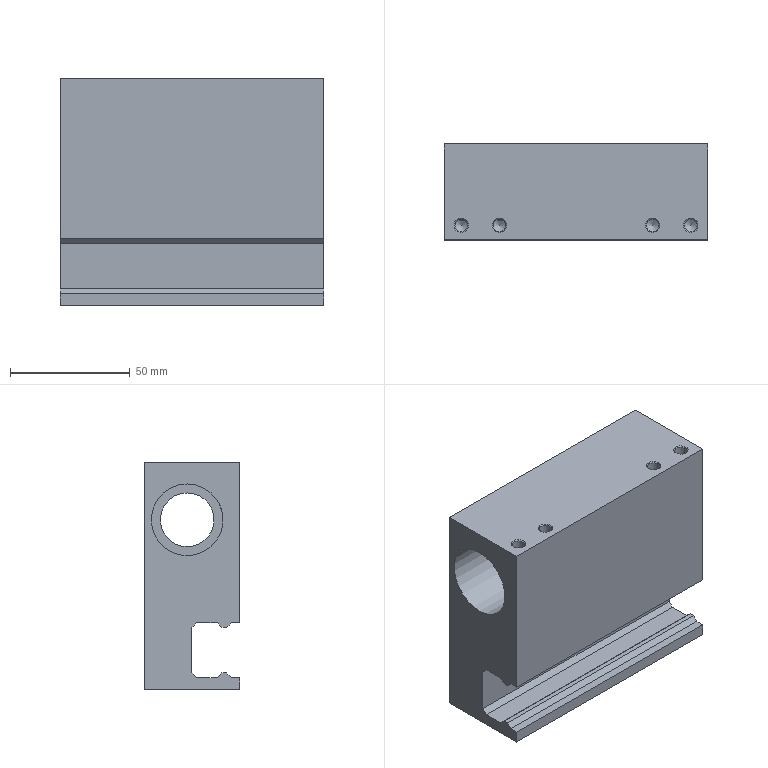Part | NX | features SIMPLE HOLE 14, SYMBOLIC_THREAD 13, DATUM_CSYS 6, HOLE PACKAGE 5, SKETCH 5, EXTRUDE 2, SUBTRACT 1 | 1 solid | 61 faces | box 110 x 40 x 95 mm | volume 303623 mm3 | cone 24 | plane 22 | cylinder 15 | commonest cylinder face diameters 5.2 x12 22.5 x1 29 x1 30 x1
STEP:
#1=CARTESIAN_POINT('',(-55.,-3.5,11.5));
#2=VERTEX_POINT('',#1);
#3=CARTESIAN_POINT('',(55.,-3.5,11.5));
#4=VERTEX_POINT('',#3);
#5=CARTESIAN_POINT('',(55.,-3.5,11.5));
#6=DIRECTION('',(-1.,0.,0.));
#7=VECTOR('',#6,1000.);
#8=LINE('',#5,#7);
#9=EDGE_CURVE('',#2,#4,#8,.F.);
#10=ORIENTED_EDGE('',*,*,#9,.T.);
#11=CARTESIAN_POINT('',(55.,-3.5,78.5));
#12=VERTEX_POINT('',#11);
#13=CARTESIAN_POINT('',(55.,-3.5,78.5));
#14=DIRECTION('',(0.,0.,-1.));
#15=VECTOR('',#14,1000.);
#16=LINE('',#13,#15);
#17=EDGE_CURVE('',#12,#4,#16,.T.);
#18=ORIENTED_EDGE('',*,*,#17,.F.);
#19=CARTESIAN_POINT('',(-55.,-3.5,78.5));
#20=VERTEX_POINT('',#19);
#21=CARTESIAN_POINT('',(55.,-3.5,78.5));
#22=DIRECTION('',(-1.,0.,0.));
#23=VECTOR('',#22,1000.);
#24=LINE('',#21,#23);
#25=EDGE_CURVE('',#12,#20,#24,.T.);
#26=ORIENTED_EDGE('',*,*,#25,.T.);
#27=CARTESIAN_POINT('',(-55.,-3.5,78.5));
#28=DIRECTION('',(0.,0.,-1.));
#29=VECTOR('',#28,1000.);
#30=LINE('',#27,#29);
#31=EDGE_CURVE('',#20,#2,#30,.T.);
#32=ORIENTED_EDGE('',*,*,#31,.T.);
#33=EDGE_LOOP('',(#10,#18,#26,#32));
#34=FACE_BOUND('',#33,.T.);
#35=CARTESIAN_POINT('',(55.,-3.5,78.5));
#36=DIRECTION('',(0.,1.,0.));
#37=DIRECTION('',(0.,0.,1.));
#38=AXIS2_PLACEMENT_3D('',#35,#36,#37);
#39=PLANE('',#38);
#40=ADVANCED_FACE('',(#34),#39,.F.);
#41=CARTESIAN_POINT('',(55.,-3.5,-11.5));
#42=VERTEX_POINT('',#41);
#43=CARTESIAN_POINT('',(-55.,-3.5,-11.5));
#44=VERTEX_POINT('',#43);
#45=CARTESIAN_POINT('',(55.,-3.5,-11.5));
#46=DIRECTION('',(1.,0.,0.));
#47=VECTOR('',#46,1000.);
#48=LINE('',#45,#47);
#49=EDGE_CURVE('',#42,#44,#48,.F.);
#50=ORIENTED_EDGE('',*,*,#49,.T.);
#51=CARTESIAN_POINT('',(-55.,-3.5,-16.5));
#52=VERTEX_POINT('',#51);
#53=CARTESIAN_POINT('',(-55.,-3.5,78.5));
#54=DIRECTION('',(0.,0.,-1.));
#55=VECTOR('',#54,1000.);
#56=LINE('',#53,#55);
#57=EDGE_CURVE('',#44,#52,#56,.T.);
#58=ORIENTED_EDGE('',*,*,#57,.T.);
#59=CARTESIAN_POINT('',(55.,-3.5,-16.5));
#60=VERTEX_POINT('',#59);
#61=CARTESIAN_POINT('',(55.,-3.5,-16.5));
#62=DIRECTION('',(-1.,0.,0.));
#63=VECTOR('',#62,1000.);
#64=LINE('',#61,#63);
#65=EDGE_CURVE('',#60,#52,#64,.T.);
#66=ORIENTED_EDGE('',*,*,#65,.F.);
#67=CARTESIAN_POINT('',(55.,-3.5,78.5));
#68=DIRECTION('',(0.,0.,-1.));
#69=VECTOR('',#68,1000.);
#70=LINE('',#67,#69);
#71=EDGE_CURVE('',#42,#60,#70,.T.);
#72=ORIENTED_EDGE('',*,*,#71,.F.);
#73=EDGE_LOOP('',(#50,#58,#66,#72));
#74=FACE_BOUND('',#73,.T.);
#75=CARTESIAN_POINT('',(55.,-3.5,78.5));
#76=DIRECTION('',(0.,1.,0.));
#77=DIRECTION('',(0.,0.,1.));
#78=AXIS2_PLACEMENT_3D('',#75,#76,#77);
#79=PLANE('',#78);
#80=ADVANCED_FACE('',(#74),#79,.F.);
#81=CARTESIAN_POINT('',(55.,18.5,69.));
#82=VERTEX_POINT('',#81);
#83=CARTESIAN_POINT('',(55.,18.5,54.5));
#84=DIRECTION('',(-1.,0.,0.));
#85=DIRECTION('',(0.,0.,1.));
#86=AXIS2_PLACEMENT_3D('',#83,#84,#85);
#87=CIRCLE('',#86,14.5);
#88=EDGE_CURVE('',#82,#82,#87,.T.);
#89=ORIENTED_EDGE('',*,*,#88,.T.);
#90=EDGE_LOOP('',(#89));
#91=FACE_BOUND('',#90,.T.);
#92=ORIENTED_EDGE('',*,*,#17,.T.);
#93=CARTESIAN_POINT('',(55.,0.,11.5));
#94=VERTEX_POINT('',#93);
#95=CARTESIAN_POINT('',(55.,18.5,11.5));
#96=DIRECTION('',(0.,1.,0.));
#97=VECTOR('',#96,1000.);
#98=LINE('',#95,#97);
#99=EDGE_CURVE('',#94,#4,#98,.F.);
#100=ORIENTED_EDGE('',*,*,#99,.F.);
#101=CARTESIAN_POINT('',(55.,2.,9.5));
#102=VERTEX_POINT('',#101);
#103=CARTESIAN_POINT('',(55.,-12.25,23.75));
#104=DIRECTION('',(0.,0.7071,-0.7071));
#105=VECTOR('',#104,1000.);
#106=LINE('',#103,#105);
#107=EDGE_CURVE('',#102,#94,#106,.F.);
#108=ORIENTED_EDGE('',*,*,#107,.F.);
#109=CARTESIAN_POINT('',(55.,4.,9.5));
#110=VERTEX_POINT('',#109);
#111=CARTESIAN_POINT('',(55.,18.5,9.5));
#112=DIRECTION('',(0.,1.,0.));
#113=VECTOR('',#112,1000.);
#114=LINE('',#111,#113);
#115=EDGE_CURVE('',#110,#102,#114,.F.);
#116=ORIENTED_EDGE('',*,*,#115,.F.);
#117=CARTESIAN_POINT('',(55.,6.,11.5));
#118=VERTEX_POINT('',#117);
#119=CARTESIAN_POINT('',(55.,33.75,39.25));
#120=DIRECTION('',(0.,0.7071,0.7071));
#121=VECTOR('',#120,1000.);
#122=LINE('',#119,#121);
#123=EDGE_CURVE('',#118,#110,#122,.F.);
#124=ORIENTED_EDGE('',*,*,#123,.F.);
#125=CARTESIAN_POINT('',(55.,14.5,11.5));
#126=VERTEX_POINT('',#125);
#127=CARTESIAN_POINT('',(55.,18.5,11.5));
#128=DIRECTION('',(0.,1.,0.));
#129=VECTOR('',#128,1000.);
#130=LINE('',#127,#129);
#131=EDGE_CURVE('',#126,#118,#130,.F.);
#132=ORIENTED_EDGE('',*,*,#131,.F.);
#133=CARTESIAN_POINT('',(55.,16.5,9.5));
#134=VERTEX_POINT('',#133);
#135=CARTESIAN_POINT('',(55.,-5.,31.));
#136=DIRECTION('',(0.,0.7071,-0.7071));
#137=VECTOR('',#136,1000.);
#138=LINE('',#135,#137);
#139=EDGE_CURVE('',#134,#126,#138,.F.);
#140=ORIENTED_EDGE('',*,*,#139,.F.);
#141=CARTESIAN_POINT('',(55.,16.5,-9.5));
#142=VERTEX_POINT('',#141);
#143=CARTESIAN_POINT('',(55.,16.5,54.5));
#144=DIRECTION('',(0.,0.,-1.));
#145=VECTOR('',#144,1000.);
#146=LINE('',#143,#145);
#147=EDGE_CURVE('',#142,#134,#146,.F.);
#148=ORIENTED_EDGE('',*,*,#147,.F.);
#149=CARTESIAN_POINT('',(55.,14.5,-11.5));
#150=VERTEX_POINT('',#149);
#151=CARTESIAN_POINT('',(55.,49.5,23.5));
#152=DIRECTION('',(0.,-0.7071,-0.7071));
#153=VECTOR('',#152,1000.);
#154=LINE('',#151,#153);
#155=EDGE_CURVE('',#150,#142,#154,.F.);
#156=ORIENTED_EDGE('',*,*,#155,.F.);
#157=CARTESIAN_POINT('',(55.,6.,-11.5));
#158=VERTEX_POINT('',#157);
#159=CARTESIAN_POINT('',(55.,18.5,-11.5));
#160=DIRECTION('',(0.,-1.,0.));
#161=VECTOR('',#160,1000.);
#162=LINE('',#159,#161);
#163=EDGE_CURVE('',#158,#150,#162,.F.);
#164=ORIENTED_EDGE('',*,*,#163,.F.);
#165=CARTESIAN_POINT('',(55.,4.,-9.5));
#166=VERTEX_POINT('',#165);
#167=CARTESIAN_POINT('',(55.,-20.75,15.25));
#168=DIRECTION('',(0.,-0.7071,0.7071));
#169=VECTOR('',#168,1000.);
#170=LINE('',#167,#169);
#171=EDGE_CURVE('',#166,#158,#170,.F.);
#172=ORIENTED_EDGE('',*,*,#171,.F.);
#173=CARTESIAN_POINT('',(55.,2.,-9.5));
#174=VERTEX_POINT('',#173);
#175=CARTESIAN_POINT('',(55.,18.5,-9.5));
#176=DIRECTION('',(0.,-1.,0.));
#177=VECTOR('',#176,1000.);
#178=LINE('',#175,#177);
#179=EDGE_CURVE('',#174,#166,#178,.F.);
#180=ORIENTED_EDGE('',*,*,#179,.F.);
#181=CARTESIAN_POINT('',(55.,0.,-11.5));
#182=VERTEX_POINT('',#181);
#183=CARTESIAN_POINT('',(55.,42.25,30.75));
#184=DIRECTION('',(0.,-0.7071,-0.7071));
#185=VECTOR('',#184,1000.);
#186=LINE('',#183,#185);
#187=EDGE_CURVE('',#182,#174,#186,.F.);
#188=ORIENTED_EDGE('',*,*,#187,.F.);
#189=CARTESIAN_POINT('',(55.,18.5,-11.5));
#190=DIRECTION('',(0.,-1.,0.));
#191=VECTOR('',#190,1000.);
#192=LINE('',#189,#191);
#193=EDGE_CURVE('',#42,#182,#192,.F.);
#194=ORIENTED_EDGE('',*,*,#193,.F.);
#195=ORIENTED_EDGE('',*,*,#71,.T.);
#196=CARTESIAN_POINT('',(55.,36.5,-16.5));
#197=VERTEX_POINT('',#196);
#198=CARTESIAN_POINT('',(55.,-3.5,-16.5));
#199=DIRECTION('',(0.,1.,0.));
#200=VECTOR('',#199,1000.);
#201=LINE('',#198,#200);
#202=EDGE_CURVE('',#60,#197,#201,.T.);
#203=ORIENTED_EDGE('',*,*,#202,.T.);
#204=CARTESIAN_POINT('',(55.,36.5,78.5));
#205=VERTEX_POINT('',#204);
#206=CARTESIAN_POINT('',(55.,36.5,-16.5));
#207=DIRECTION('',(0.,0.,1.));
#208=VECTOR('',#207,1000.);
#209=LINE('',#206,#208);
#210=EDGE_CURVE('',#197,#205,#209,.T.);
#211=ORIENTED_EDGE('',*,*,#210,.T.);
#212=CARTESIAN_POINT('',(55.,36.5,78.5));
#213=DIRECTION('',(0.,-1.,0.));
#214=VECTOR('',#213,1000.);
#215=LINE('',#212,#214);
#216=EDGE_CURVE('',#205,#12,#215,.T.);
#217=ORIENTED_EDGE('',*,*,#216,.T.);
#218=EDGE_LOOP('',(#92,#100,#108,#116,#124,#132,#140,#148,#156,#164,#172,#180,#188,#194,#195,#203,#211,#217));
#219=FACE_BOUND('',#218,.T.);
#220=CARTESIAN_POINT('',(55.,18.5,54.5));
#221=DIRECTION('',(1.,0.,0.));
#222=DIRECTION('',(0.,0.,-1.));
#223=AXIS2_PLACEMENT_3D('',#220,#221,#222);
#224=PLANE('',#223);
#225=ADVANCED_FACE('',(#91,#219),#224,.T.);
#226=CARTESIAN_POINT('',(-55.,18.5,39.5));
#227=VERTEX_POINT('',#226);
#228=CARTESIAN_POINT('',(-55.,18.5,54.5));
#229=DIRECTION('',(1.,0.,0.));
#230=DIRECTION('',(0.,0.,-1.));
#231=AXIS2_PLACEMENT_3D('',#228,#229,#230);
#232=CIRCLE('',#231,15.);
#233=EDGE_CURVE('',#227,#227,#232,.T.);
#234=ORIENTED_EDGE('',*,*,#233,.T.);
#235=EDGE_LOOP('',(#234));
#236=FACE_BOUND('',#235,.T.);
#237=CARTESIAN_POINT('',(-55.,0.,11.5));
#238=VERTEX_POINT('',#237);
#239=CARTESIAN_POINT('',(-55.,18.5,11.5));
#240=DIRECTION('',(0.,1.,0.));
#241=VECTOR('',#240,1000.);
#242=LINE('',#239,#241);
#243=EDGE_CURVE('',#238,#2,#242,.F.);
#244=ORIENTED_EDGE('',*,*,#243,.T.);
#245=ORIENTED_EDGE('',*,*,#31,.F.);
#246=CARTESIAN_POINT('',(-55.,36.5,78.5));
#247=VERTEX_POINT('',#246);
#248=CARTESIAN_POINT('',(-55.,36.5,78.5));
#249=DIRECTION('',(0.,-1.,0.));
#250=VECTOR('',#249,1000.);
#251=LINE('',#248,#250);
#252=EDGE_CURVE('',#247,#20,#251,.T.);
#253=ORIENTED_EDGE('',*,*,#252,.F.);
#254=CARTESIAN_POINT('',(-55.,36.5,-16.5));
#255=VERTEX_POINT('',#254);
#256=CARTESIAN_POINT('',(-55.,36.5,-16.5));
#257=DIRECTION('',(0.,0.,1.));
#258=VECTOR('',#257,1000.);
#259=LINE('',#256,#258);
#260=EDGE_CURVE('',#255,#247,#259,.T.);
#261=ORIENTED_EDGE('',*,*,#260,.F.);
#262=CARTESIAN_POINT('',(-55.,-3.5,-16.5));
#263=DIRECTION('',(0.,1.,0.));
#264=VECTOR('',#263,1000.);
#265=LINE('',#262,#264);
#266=EDGE_CURVE('',#52,#255,#265,.T.);
#267=ORIENTED_EDGE('',*,*,#266,.F.);
#268=ORIENTED_EDGE('',*,*,#57,.F.);
#269=CARTESIAN_POINT('',(-55.,0.,-11.5));
#270=VERTEX_POINT('',#269);
#271=CARTESIAN_POINT('',(-55.,18.5,-11.5));
#272=DIRECTION('',(0.,-1.,0.));
#273=VECTOR('',#272,1000.);
#274=LINE('',#271,#273);
#275=EDGE_CURVE('',#44,#270,#274,.F.);
#276=ORIENTED_EDGE('',*,*,#275,.T.);
#277=CARTESIAN_POINT('',(-55.,2.,-9.5));
#278=VERTEX_POINT('',#277);
#279=CARTESIAN_POINT('',(-55.,42.25,30.75));
#280=DIRECTION('',(0.,-0.7071,-0.7071));
#281=VECTOR('',#280,1000.);
#282=LINE('',#279,#281);
#283=EDGE_CURVE('',#270,#278,#282,.F.);
#284=ORIENTED_EDGE('',*,*,#283,.T.);
#285=CARTESIAN_POINT('',(-55.,4.,-9.5));
#286=VERTEX_POINT('',#285);
#287=CARTESIAN_POINT('',(-55.,18.5,-9.5));
#288=DIRECTION('',(0.,-1.,0.));
#289=VECTOR('',#288,1000.);
#290=LINE('',#287,#289);
#291=EDGE_CURVE('',#278,#286,#290,.F.);
#292=ORIENTED_EDGE('',*,*,#291,.T.);
#293=CARTESIAN_POINT('',(-55.,6.,-11.5));
#294=VERTEX_POINT('',#293);
#295=CARTESIAN_POINT('',(-55.,-20.75,15.25));
#296=DIRECTION('',(0.,-0.7071,0.7071));
#297=VECTOR('',#296,1000.);
#298=LINE('',#295,#297);
#299=EDGE_CURVE('',#286,#294,#298,.F.);
#300=ORIENTED_EDGE('',*,*,#299,.T.);
#301=CARTESIAN_POINT('',(-55.,14.5,-11.5));
#302=VERTEX_POINT('',#301);
#303=CARTESIAN_POINT('',(-55.,18.5,-11.5));
#304=DIRECTION('',(0.,-1.,0.));
#305=VECTOR('',#304,1000.);
#306=LINE('',#303,#305);
#307=EDGE_CURVE('',#294,#302,#306,.F.);
#308=ORIENTED_EDGE('',*,*,#307,.T.);
#309=CARTESIAN_POINT('',(-55.,16.5,-9.5));
#310=VERTEX_POINT('',#309);
#311=CARTESIAN_POINT('',(-55.,49.5,23.5));
#312=DIRECTION('',(0.,-0.7071,-0.7071));
#313=VECTOR('',#312,1000.);
#314=LINE('',#311,#313);
#315=EDGE_CURVE('',#302,#310,#314,.F.);
#316=ORIENTED_EDGE('',*,*,#315,.T.);
#317=CARTESIAN_POINT('',(-55.,16.5,9.5));
#318=VERTEX_POINT('',#317);
#319=CARTESIAN_POINT('',(-55.,16.5,54.5));
#320=DIRECTION('',(0.,0.,-1.));
#321=VECTOR('',#320,1000.);
#322=LINE('',#319,#321);
#323=EDGE_CURVE('',#310,#318,#322,.F.);
#324=ORIENTED_EDGE('',*,*,#323,.T.);
#325=CARTESIAN_POINT('',(-55.,14.5,11.5));
#326=VERTEX_POINT('',#325);
#327=CARTESIAN_POINT('',(-55.,-5.,31.));
#328=DIRECTION('',(0.,0.7071,-0.7071));
#329=VECTOR('',#328,1000.);
#330=LINE('',#327,#329);
#331=EDGE_CURVE('',#318,#326,#330,.F.);
#332=ORIENTED_EDGE('',*,*,#331,.T.);
#333=CARTESIAN_POINT('',(-55.,6.,11.5));
#334=VERTEX_POINT('',#333);
#335=CARTESIAN_POINT('',(-55.,18.5,11.5));
#336=DIRECTION('',(0.,1.,0.));
#337=VECTOR('',#336,1000.);
#338=LINE('',#335,#337);
#339=EDGE_CURVE('',#326,#334,#338,.F.);
#340=ORIENTED_EDGE('',*,*,#339,.T.);
#341=CARTESIAN_POINT('',(-55.,4.,9.5));
#342=VERTEX_POINT('',#341);
#343=CARTESIAN_POINT('',(-55.,33.75,39.25));
#344=DIRECTION('',(0.,0.7071,0.7071));
#345=VECTOR('',#344,1000.);
#346=LINE('',#343,#345);
#347=EDGE_CURVE('',#334,#342,#346,.F.);
#348=ORIENTED_EDGE('',*,*,#347,.T.);
#349=CARTESIAN_POINT('',(-55.,2.,9.5));
#350=VERTEX_POINT('',#349);
#351=CARTESIAN_POINT('',(-55.,18.5,9.5));
#352=DIRECTION('',(0.,1.,0.));
#353=VECTOR('',#352,1000.);
#354=LINE('',#351,#353);
#355=EDGE_CURVE('',#342,#350,#354,.F.);
#356=ORIENTED_EDGE('',*,*,#355,.T.);
#357=CARTESIAN_POINT('',(-55.,-12.25,23.75));
#358=DIRECTION('',(0.,0.7071,-0.7071));
#359=VECTOR('',#358,1000.);
#360=LINE('',#357,#359);
#361=EDGE_CURVE('',#350,#238,#360,.F.);
#362=ORIENTED_EDGE('',*,*,#361,.T.);
#363=EDGE_LOOP('',(#244,#245,#253,#261,#267,#268,#276,#284,#292,#300,#308,#316,#324,#332,#340,#348,#356,#362));
#364=FACE_BOUND('',#363,.T.);
#365=CARTESIAN_POINT('',(-55.,18.5,54.5));
#366=DIRECTION('',(1.,0.,0.));
#367=DIRECTION('',(0.,0.,-1.));
#368=AXIS2_PLACEMENT_3D('',#365,#366,#367);
#369=PLANE('',#368);
#370=ADVANCED_FACE('',(#236,#364),#369,.F.);
#371=CARTESIAN_POINT('',(43.,22.5,-16.5));
#372=VERTEX_POINT('',#371);
#373=CARTESIAN_POINT('',(40.,22.5,-16.5));
#374=DIRECTION('',(0.,0.,1.));
#375=DIRECTION('',(1.,0.,0.));
#376=AXIS2_PLACEMENT_3D('',#373,#374,#375);
#377=CIRCLE('',#376,3.);
#378=EDGE_CURVE('',#372,#372,#377,.T.);
#379=ORIENTED_EDGE('',*,*,#378,.T.);
#380=EDGE_LOOP('',(#379));
#381=FACE_BOUND('',#380,.T.);
#382=CARTESIAN_POINT('',(17.,22.5,-16.5));
#383=VERTEX_POINT('',#382);
#384=CARTESIAN_POINT('',(14.,22.5,-16.5));
#385=DIRECTION('',(0.,0.,1.));
#386=DIRECTION('',(1.,0.,0.));
#387=AXIS2_PLACEMENT_3D('',#384,#385,#386);
#388=CIRCLE('',#387,3.);
#389=EDGE_CURVE('',#383,#383,#388,.T.);
#390=ORIENTED_EDGE('',*,*,#389,.T.);
#391=EDGE_LOOP('',(#390));
#392=FACE_BOUND('',#391,.T.);
#393=CARTESIAN_POINT('',(-11.,22.5,-16.5));
#394=VERTEX_POINT('',#393);
#395=CARTESIAN_POINT('',(-14.,22.5,-16.5));
#396=DIRECTION('',(0.,0.,1.));
#397=DIRECTION('',(1.,0.,0.));
#398=AXIS2_PLACEMENT_3D('',#395,#396,#397);
#399=CIRCLE('',#398,3.);
#400=EDGE_CURVE('',#394,#394,#399,.T.);
#401=ORIENTED_EDGE('',*,*,#400,.T.);
#402=EDGE_LOOP('',(#401));
#403=FACE_BOUND('',#402,.T.);
#404=CARTESIAN_POINT('',(-37.,22.5,-16.5));
#405=VERTEX_POINT('',#404);
#406=CARTESIAN_POINT('',(-40.,22.5,-16.5));
#407=DIRECTION('',(0.,0.,1.));
#408=DIRECTION('',(1.,0.,0.));
#409=AXIS2_PLACEMENT_3D('',#406,#407,#408);
#410=CIRCLE('',#409,3.);
#411=EDGE_CURVE('',#405,#405,#410,.T.);
#412=ORIENTED_EDGE('',*,*,#411,.T.);
#413=EDGE_LOOP('',(#412));
#414=FACE_BOUND('',#413,.T.);
#415=ORIENTED_EDGE('',*,*,#266,.T.);
#416=CARTESIAN_POINT('',(55.,36.5,-16.5));
#417=DIRECTION('',(-1.,0.,0.));
#418=VECTOR('',#417,1000.);
#419=LINE('',#416,#418);
#420=EDGE_CURVE('',#197,#255,#419,.T.);
#421=ORIENTED_EDGE('',*,*,#420,.F.);
#422=ORIENTED_EDGE('',*,*,#202,.F.);
#423=ORIENTED_EDGE('',*,*,#65,.T.);
#424=EDGE_LOOP('',(#415,#421,#422,#423));
#425=FACE_BOUND('',#424,.T.);
#426=CARTESIAN_POINT('',(55.,-3.5,-16.5));
#427=DIRECTION('',(0.,0.,1.));
#428=DIRECTION('',(1.,0.,0.));
#429=AXIS2_PLACEMENT_3D('',#426,#427,#428);
#430=PLANE('',#429);
#431=ADVANCED_FACE('',(#381,#392,#403,#414,#425),#430,.F.);
#432=CARTESIAN_POINT('',(46.,36.5,33.5));
#433=VERTEX_POINT('',#432);
#434=CARTESIAN_POINT('',(46.,36.5,36.5));
#435=DIRECTION('',(0.,-1.,0.));
#436=DIRECTION('',(0.,0.,-1.));
#437=AXIS2_PLACEMENT_3D('',#434,#435,#436);
#438=CIRCLE('',#437,3.);
#439=EDGE_CURVE('',#433,#433,#438,.T.);
#440=ORIENTED_EDGE('',*,*,#439,.T.);
#441=EDGE_LOOP('',(#440));
#442=FACE_BOUND('',#441,.T.);
#443=CARTESIAN_POINT('',(46.,36.5,17.5));
#444=VERTEX_POINT('',#443);
#445=CARTESIAN_POINT('',(46.,36.5,20.5));
#446=DIRECTION('',(0.,-1.,0.));
#447=DIRECTION('',(0.,0.,-1.));
#448=AXIS2_PLACEMENT_3D('',#445,#446,#447);
#449=CIRCLE('',#448,3.);
#450=EDGE_CURVE('',#444,#444,#449,.T.);
#451=ORIENTED_EDGE('',*,*,#450,.T.);
#452=EDGE_LOOP('',(#451));
#453=FACE_BOUND('',#452,.T.);
#454=CARTESIAN_POINT('',(-16.,36.5,17.5));
#455=VERTEX_POINT('',#454);
#456=CARTESIAN_POINT('',(-16.,36.5,20.5));
#457=DIRECTION('',(0.,-1.,0.));
#458=DIRECTION('',(0.,0.,-1.));
#459=AXIS2_PLACEMENT_3D('',#456,#457,#458);
#460=CIRCLE('',#459,3.);
#461=EDGE_CURVE('',#455,#455,#460,.T.);
#462=ORIENTED_EDGE('',*,*,#461,.T.);
#463=EDGE_LOOP('',(#462));
#464=FACE_BOUND('',#463,.T.);
#465=CARTESIAN_POINT('',(-16.,36.5,33.5));
#466=VERTEX_POINT('',#465);
#467=CARTESIAN_POINT('',(-16.,36.5,36.5));
#468=DIRECTION('',(0.,-1.,0.));
#469=DIRECTION('',(0.,0.,-1.));
#470=AXIS2_PLACEMENT_3D('',#467,#468,#469);
#471=CIRCLE('',#470,3.);
#472=EDGE_CURVE('',#466,#466,#471,.T.);
#473=ORIENTED_EDGE('',*,*,#472,.T.);
#474=EDGE_LOOP('',(#473));
#475=FACE_BOUND('',#474,.T.);
#476=ORIENTED_EDGE('',*,*,#260,.T.);
#477=CARTESIAN_POINT('',(55.,36.5,78.5));
#478=DIRECTION('',(-1.,0.,0.));
#479=VECTOR('',#478,1000.);
#480=LINE('',#477,#479);
#481=EDGE_CURVE('',#205,#247,#480,.T.);
#482=ORIENTED_EDGE('',*,*,#481,.F.);
#483=ORIENTED_EDGE('',*,*,#210,.F.);
#484=ORIENTED_EDGE('',*,*,#420,.T.);
#485=EDGE_LOOP('',(#476,#482,#483,#484));
#486=FACE_BOUND('',#485,.T.);
#487=CARTESIAN_POINT('',(55.,36.5,-16.5));
#488=DIRECTION('',(0.,-1.,0.));
#489=DIRECTION('',(0.,0.,-1.));
#490=AXIS2_PLACEMENT_3D('',#487,#488,#489);
#491=PLANE('',#490);
#492=ADVANCED_FACE('',(#442,#453,#464,#475,#486),#491,.F.);
#493=CARTESIAN_POINT('',(45.,2.5,78.5));
#494=VERTEX_POINT('',#493);
#495=CARTESIAN_POINT('',(48.,2.5,78.5));
#496=DIRECTION('',(0.,0.,-1.));
#497=DIRECTION('',(-1.,0.,0.));
#498=AXIS2_PLACEMENT_3D('',#495,#496,#497);
#499=CIRCLE('',#498,3.);
#500=EDGE_CURVE('',#494,#494,#499,.T.);
#501=ORIENTED_EDGE('',*,*,#500,.T.);
#502=EDGE_LOOP('',(#501));
#503=FACE_BOUND('',#502,.T.);
#504=CARTESIAN_POINT('',(29.,2.5,78.5));
#505=VERTEX_POINT('',#504);
#506=CARTESIAN_POINT('',(32.,2.5,78.5));
#507=DIRECTION('',(0.,0.,-1.));
#508=DIRECTION('',(-1.,0.,0.));
#509=AXIS2_PLACEMENT_3D('',#506,#507,#508);
#510=CIRCLE('',#509,3.);
#511=EDGE_CURVE('',#505,#505,#510,.T.);
#512=ORIENTED_EDGE('',*,*,#511,.T.);
#513=EDGE_LOOP('',(#512));
#514=FACE_BOUND('',#513,.T.);
#515=CARTESIAN_POINT('',(-35.,2.5,78.5));
#516=VERTEX_POINT('',#515);
#517=CARTESIAN_POINT('',(-32.,2.5,78.5));
#518=DIRECTION('',(0.,0.,-1.));
#519=DIRECTION('',(-1.,0.,0.));
#520=AXIS2_PLACEMENT_3D('',#517,#518,#519);
#521=CIRCLE('',#520,3.);
#522=EDGE_CURVE('',#516,#516,#521,.T.);
#523=ORIENTED_EDGE('',*,*,#522,.T.);
#524=EDGE_LOOP('',(#523));
#525=FACE_BOUND('',#524,.T.);
#526=CARTESIAN_POINT('',(-51.,2.5,78.5));
#527=VERTEX_POINT('',#526);
#528=CARTESIAN_POINT('',(-48.,2.5,78.5));
#529=DIRECTION('',(0.,0.,-1.));
#530=DIRECTION('',(-1.,0.,0.));
#531=AXIS2_PLACEMENT_3D('',#528,#529,#530);
#532=CIRCLE('',#531,3.);
#533=EDGE_CURVE('',#527,#527,#532,.T.);
#534=ORIENTED_EDGE('',*,*,#533,.T.);
#535=EDGE_LOOP('',(#534));
#536=FACE_BOUND('',#535,.T.);
#537=ORIENTED_EDGE('',*,*,#252,.T.);
#538=ORIENTED_EDGE('',*,*,#25,.F.);
#539=ORIENTED_EDGE('',*,*,#216,.F.);
#540=ORIENTED_EDGE('',*,*,#481,.T.);
#541=EDGE_LOOP('',(#537,#538,#539,#540));
#542=FACE_BOUND('',#541,.T.);
#543=CARTESIAN_POINT('',(55.,36.5,78.5));
#544=DIRECTION('',(0.,0.,-1.));
#545=DIRECTION('',(-1.,0.,0.));
#546=AXIS2_PLACEMENT_3D('',#543,#544,#545);
#547=PLANE('',#546);
#548=ADVANCED_FACE('',(#503,#514,#525,#536,#542),#547,.F.);
#549=CARTESIAN_POINT('',(-25.,18.5,43.25));
#550=VERTEX_POINT('',#549);
#551=CARTESIAN_POINT('',(-25.,18.5,54.5));
#552=DIRECTION('',(1.,0.,0.));
#553=DIRECTION('',(0.,0.,-1.));
#554=AXIS2_PLACEMENT_3D('',#551,#552,#553);
#555=CIRCLE('',#554,11.25);
#556=EDGE_CURVE('',#550,#550,#555,.T.);
#557=ORIENTED_EDGE('',*,*,#556,.F.);
#558=EDGE_LOOP('',(#557));
#559=FACE_BOUND('',#558,.T.);
#560=CARTESIAN_POINT('',(25.,18.5,65.75));
#561=VERTEX_POINT('',#560);
#562=CARTESIAN_POINT('',(25.,18.5,54.5));
#563=DIRECTION('',(-1.,0.,0.));
#564=DIRECTION('',(0.,0.,1.));
#565=AXIS2_PLACEMENT_3D('',#562,#563,#564);
#566=CIRCLE('',#565,11.25);
#567=EDGE_CURVE('',#561,#561,#566,.T.);
#568=ORIENTED_EDGE('',*,*,#567,.F.);
#569=EDGE_LOOP('',(#568));
#570=FACE_BOUND('',#569,.T.);
#571=CARTESIAN_POINT('',(55.,18.5,54.5));
#572=DIRECTION('',(-1.,0.,0.));
#573=DIRECTION('',(0.,0.,1.));
#574=AXIS2_PLACEMENT_3D('',#571,#572,#573);
#575=CYLINDRICAL_SURFACE('',#574,11.25);
#576=ADVANCED_FACE('',(#559,#570),#575,.F.);
#577=CARTESIAN_POINT('',(225.,2.,-9.5));
#578=DIRECTION('',(-1.,0.,0.));
#579=VECTOR('',#578,1000.);
#580=LINE('',#577,#579);
#581=EDGE_CURVE('',#278,#174,#580,.F.);
#582=ORIENTED_EDGE('',*,*,#581,.F.);
#583=ORIENTED_EDGE('',*,*,#283,.F.);
#584=CARTESIAN_POINT('',(225.,0.,-11.5));
#585=DIRECTION('',(-1.,0.,0.));
#586=VECTOR('',#585,1000.);
#587=LINE('',#584,#586);
#588=EDGE_CURVE('',#270,#182,#587,.F.);
#589=ORIENTED_EDGE('',*,*,#588,.T.);
#590=ORIENTED_EDGE('',*,*,#187,.T.);
#591=EDGE_LOOP('',(#582,#583,#589,#590));
#592=FACE_BOUND('',#591,.T.);
#593=CARTESIAN_POINT('',(225.,0.,-11.5));
#594=DIRECTION('',(0.,-0.7071,0.7071));
#595=DIRECTION('',(0.,-0.7071,-0.7071));
#596=AXIS2_PLACEMENT_3D('',#593,#594,#595);
#597=PLANE('',#596);
#598=ADVANCED_FACE('',(#592),#597,.T.);
#599=CARTESIAN_POINT('',(225.,4.,-9.5));
#600=DIRECTION('',(-1.,0.,0.));
#601=VECTOR('',#600,1000.);
#602=LINE('',#599,#601);
#603=EDGE_CURVE('',#286,#166,#602,.F.);
#604=ORIENTED_EDGE('',*,*,#603,.F.);
#605=ORIENTED_EDGE('',*,*,#291,.F.);
#606=ORIENTED_EDGE('',*,*,#581,.T.);
#607=ORIENTED_EDGE('',*,*,#179,.T.);
#608=EDGE_LOOP('',(#604,#605,#606,#607));
#609=FACE_BOUND('',#608,.T.);
#610=CARTESIAN_POINT('',(225.,2.,-9.5));
#611=DIRECTION('',(0.,0.,1.));
#612=DIRECTION('',(1.,0.,0.));
#613=AXIS2_PLACEMENT_3D('',#610,#611,#612);
#614=PLANE('',#613);
#615=ADVANCED_FACE('',(#609),#614,.T.);
#616=CARTESIAN_POINT('',(225.,6.,-11.5));
#617=DIRECTION('',(-1.,0.,0.));
#618=VECTOR('',#617,1000.);
#619=LINE('',#616,#618);
#620=EDGE_CURVE('',#294,#158,#619,.F.);
#621=ORIENTED_EDGE('',*,*,#620,.F.);
#622=ORIENTED_EDGE('',*,*,#299,.F.);
#623=ORIENTED_EDGE('',*,*,#603,.T.);
#624=ORIENTED_EDGE('',*,*,#171,.T.);
#625=EDGE_LOOP('',(#621,#622,#623,#624));
#626=FACE_BOUND('',#625,.T.);
#627=CARTESIAN_POINT('',(225.,4.,-9.5));
#628=DIRECTION('',(0.,0.7071,0.7071));
#629=DIRECTION('',(0.,-0.7071,0.7071));
#630=AXIS2_PLACEMENT_3D('',#627,#628,#629);
#631=PLANE('',#630);
#632=ADVANCED_FACE('',(#626),#631,.T.);
#633=CARTESIAN_POINT('',(225.,14.5,-11.5));
#634=DIRECTION('',(-1.,0.,0.));
#635=VECTOR('',#634,1000.);
#636=LINE('',#633,#635);
#637=EDGE_CURVE('',#302,#150,#636,.F.);
#638=ORIENTED_EDGE('',*,*,#637,.F.);
#639=ORIENTED_EDGE('',*,*,#307,.F.);
#640=ORIENTED_EDGE('',*,*,#620,.T.);
#641=ORIENTED_EDGE('',*,*,#163,.T.);
#642=EDGE_LOOP('',(#638,#639,#640,#641));
#643=FACE_BOUND('',#642,.T.);
#644=CARTESIAN_POINT('',(225.,6.,-11.5));
#645=DIRECTION('',(0.,0.,1.));
#646=DIRECTION('',(0.,-1.,0.));
#647=AXIS2_PLACEMENT_3D('',#644,#645,#646);
#648=PLANE('',#647);
#649=ADVANCED_FACE('',(#643),#648,.T.);
#650=CARTESIAN_POINT('',(225.,16.5,-9.5));
#651=DIRECTION('',(-1.,0.,0.));
#652=VECTOR('',#651,1000.);
#653=LINE('',#650,#652);
#654=EDGE_CURVE('',#310,#142,#653,.F.);
#655=ORIENTED_EDGE('',*,*,#654,.F.);
#656=ORIENTED_EDGE('',*,*,#315,.F.);
#657=ORIENTED_EDGE('',*,*,#637,.T.);
#658=ORIENTED_EDGE('',*,*,#155,.T.);
#659=EDGE_LOOP('',(#655,#656,#657,#658));
#660=FACE_BOUND('',#659,.T.);
#661=CARTESIAN_POINT('',(225.,14.5,-11.5));
#662=DIRECTION('',(0.,-0.7071,0.7071));
#663=DIRECTION('',(0.,-0.7071,-0.7071));
#664=AXIS2_PLACEMENT_3D('',#661,#662,#663);
#665=PLANE('',#664);
#666=ADVANCED_FACE('',(#660),#665,.T.);
#667=CARTESIAN_POINT('',(225.,16.5,9.5));
#668=DIRECTION('',(-1.,0.,0.));
#669=VECTOR('',#668,1000.);
#670=LINE('',#667,#669);
#671=EDGE_CURVE('',#318,#134,#670,.F.);
#672=ORIENTED_EDGE('',*,*,#671,.F.);
#673=ORIENTED_EDGE('',*,*,#323,.F.);
#674=ORIENTED_EDGE('',*,*,#654,.T.);
#675=ORIENTED_EDGE('',*,*,#147,.T.);
#676=EDGE_LOOP('',(#672,#673,#674,#675));
#677=FACE_BOUND('',#676,.T.);
#678=CARTESIAN_POINT('',(225.,16.5,0.));
#679=DIRECTION('',(0.,-1.,0.));
#680=DIRECTION('',(0.,0.,-1.));
#681=AXIS2_PLACEMENT_3D('',#678,#679,#680);
#682=PLANE('',#681);
#683=ADVANCED_FACE('',(#677),#682,.T.);
#684=CARTESIAN_POINT('',(225.,14.5,11.5));
#685=DIRECTION('',(-1.,0.,0.));
#686=VECTOR('',#685,1000.);
#687=LINE('',#684,#686);
#688=EDGE_CURVE('',#326,#126,#687,.F.);
#689=ORIENTED_EDGE('',*,*,#688,.F.);
#690=ORIENTED_EDGE('',*,*,#331,.F.);
#691=ORIENTED_EDGE('',*,*,#671,.T.);
#692=ORIENTED_EDGE('',*,*,#139,.T.);
#693=EDGE_LOOP('',(#689,#690,#691,#692));
#694=FACE_BOUND('',#693,.T.);
#695=CARTESIAN_POINT('',(225.,16.5,9.5));
#696=DIRECTION('',(0.,-0.7071,-0.7071));
#697=DIRECTION('',(0.,0.7071,-0.7071));
#698=AXIS2_PLACEMENT_3D('',#695,#696,#697);
#699=PLANE('',#698);
#700=ADVANCED_FACE('',(#694),#699,.T.);
#701=CARTESIAN_POINT('',(225.,6.,11.5));
#702=DIRECTION('',(-1.,0.,0.));
#703=VECTOR('',#702,1000.);
#704=LINE('',#701,#703);
#705=EDGE_CURVE('',#334,#118,#704,.F.);
#706=ORIENTED_EDGE('',*,*,#705,.F.);
#707=ORIENTED_EDGE('',*,*,#339,.F.);
#708=ORIENTED_EDGE('',*,*,#688,.T.);
#709=ORIENTED_EDGE('',*,*,#131,.T.);
#710=EDGE_LOOP('',(#706,#707,#708,#709));
#711=FACE_BOUND('',#710,.T.);
#712=CARTESIAN_POINT('',(225.,14.5,11.5));
#713=DIRECTION('',(0.,0.,-1.));
#714=DIRECTION('',(0.,1.,0.));
#715=AXIS2_PLACEMENT_3D('',#712,#713,#714);
#716=PLANE('',#715);
#717=ADVANCED_FACE('',(#711),#716,.T.);
#718=CARTESIAN_POINT('',(225.,4.,9.5));
#719=DIRECTION('',(-1.,0.,0.));
#720=VECTOR('',#719,1000.);
#721=LINE('',#718,#720);
#722=EDGE_CURVE('',#342,#110,#721,.F.);
#723=ORIENTED_EDGE('',*,*,#722,.F.);
#724=ORIENTED_EDGE('',*,*,#347,.F.);
#725=ORIENTED_EDGE('',*,*,#705,.T.);
#726=ORIENTED_EDGE('',*,*,#123,.T.);
#727=EDGE_LOOP('',(#723,#724,#725,#726));
#728=FACE_BOUND('',#727,.T.);
#729=CARTESIAN_POINT('',(225.,6.,11.5));
#730=DIRECTION('',(0.,0.7071,-0.7071));
#731=DIRECTION('',(0.,0.7071,0.7071));
#732=AXIS2_PLACEMENT_3D('',#729,#730,#731);
#733=PLANE('',#732);
#734=ADVANCED_FACE('',(#728),#733,.T.);
#735=CARTESIAN_POINT('',(225.,2.,9.5));
#736=DIRECTION('',(-1.,0.,0.));
#737=VECTOR('',#736,1000.);
#738=LINE('',#735,#737);
#739=EDGE_CURVE('',#350,#102,#738,.F.);
#740=ORIENTED_EDGE('',*,*,#739,.F.);
#741=ORIENTED_EDGE('',*,*,#355,.F.);
#742=ORIENTED_EDGE('',*,*,#722,.T.);
#743=ORIENTED_EDGE('',*,*,#115,.T.);
#744=EDGE_LOOP('',(#740,#741,#742,#743));
#745=FACE_BOUND('',#744,.T.);
#746=CARTESIAN_POINT('',(225.,4.,9.5));
#747=DIRECTION('',(0.,0.,-1.));
#748=DIRECTION('',(-1.,0.,0.));
#749=AXIS2_PLACEMENT_3D('',#746,#747,#748);
#750=PLANE('',#749);
#751=ADVANCED_FACE('',(#745),#750,.T.);
#752=CARTESIAN_POINT('',(225.,0.,11.5));
#753=DIRECTION('',(-1.,0.,0.));
#754=VECTOR('',#753,1000.);
#755=LINE('',#752,#754);
#756=EDGE_CURVE('',#238,#94,#755,.F.);
#757=ORIENTED_EDGE('',*,*,#756,.F.);
#758=ORIENTED_EDGE('',*,*,#361,.F.);
#759=ORIENTED_EDGE('',*,*,#739,.T.);
#760=ORIENTED_EDGE('',*,*,#107,.T.);
#761=EDGE_LOOP('',(#757,#758,#759,#760));
#762=FACE_BOUND('',#761,.T.);
#763=CARTESIAN_POINT('',(225.,2.,9.5));
#764=DIRECTION('',(0.,-0.7071,-0.7071));
#765=DIRECTION('',(0.,0.7071,-0.7071));
#766=AXIS2_PLACEMENT_3D('',#763,#764,#765);
#767=PLANE('',#766);
#768=ADVANCED_FACE('',(#762),#767,.T.);
#769=ORIENTED_EDGE('',*,*,#9,.F.);
#770=ORIENTED_EDGE('',*,*,#243,.F.);
#771=ORIENTED_EDGE('',*,*,#756,.T.);
#772=ORIENTED_EDGE('',*,*,#99,.T.);
#773=EDGE_LOOP('',(#769,#770,#771,#772));
#774=FACE_BOUND('',#773,.T.);
#775=CARTESIAN_POINT('',(225.,0.,11.5));
#776=DIRECTION('',(0.,0.,-1.));
#777=DIRECTION('',(0.,1.,0.));
#778=AXIS2_PLACEMENT_3D('',#775,#776,#777);
#779=PLANE('',#778);
#780=ADVANCED_FACE('',(#774),#779,.T.);
#781=ORIENTED_EDGE('',*,*,#588,.F.);
#782=ORIENTED_EDGE('',*,*,#275,.F.);
#783=ORIENTED_EDGE('',*,*,#49,.F.);
#784=ORIENTED_EDGE('',*,*,#193,.T.);
#785=EDGE_LOOP('',(#781,#782,#783,#784));
#786=FACE_BOUND('',#785,.T.);
#787=CARTESIAN_POINT('',(225.,-5.5,-11.5));
#788=DIRECTION('',(0.,0.,1.));
#789=DIRECTION('',(0.,-1.,0.));
#790=AXIS2_PLACEMENT_3D('',#787,#788,#789);
#791=PLANE('',#790);
#792=ADVANCED_FACE('',(#786),#791,.T.);
#793=CARTESIAN_POINT('',(-16.,16.5,33.9));
#794=VERTEX_POINT('',#793);
#795=CARTESIAN_POINT('',(-16.,16.5,36.5));
#796=DIRECTION('',(0.,-1.,0.));
#797=DIRECTION('',(0.,0.,-1.));
#798=AXIS2_PLACEMENT_3D('',#795,#796,#797);
#799=CIRCLE('',#798,2.6);
#800=EDGE_CURVE('',#794,#794,#799,.F.);
#801=ORIENTED_EDGE('',*,*,#800,.T.);
#802=EDGE_LOOP('',(#801));
#803=FACE_BOUND('',#802,.T.);
#804=CARTESIAN_POINT('',(-16.,14.938,36.5));
#805=VERTEX_POINT('',#804);
#806=VERTEX_LOOP('',#805);
#807=FACE_BOUND('',#806,.T.);
#808=CARTESIAN_POINT('',(-16.,16.5,36.5));
#809=DIRECTION('',(0.,1.,0.));
#810=DIRECTION('',(0.,0.,1.));
#811=AXIS2_PLACEMENT_3D('',#808,#809,#810);
#812=CONICAL_SURFACE('',#811,2.6,1.03);
#813=ADVANCED_FACE('',(#803,#807),#812,.F.);
#814=CARTESIAN_POINT('',(-16.,36.1,33.9));
#815=VERTEX_POINT('',#814);
#816=CARTESIAN_POINT('',(-16.,36.1,36.5));
#817=DIRECTION('',(0.,-1.,0.));
#818=DIRECTION('',(0.,0.,-1.));
#819=AXIS2_PLACEMENT_3D('',#816,#817,#818);
#820=CIRCLE('',#819,2.6);
#821=EDGE_CURVE('',#815,#815,#820,.F.);
#822=ORIENTED_EDGE('',*,*,#821,.T.);
#823=EDGE_LOOP('',(#822));
#824=FACE_BOUND('',#823,.T.);
#825=ORIENTED_EDGE('',*,*,#800,.F.);
#826=EDGE_LOOP('',(#825));
#827=FACE_BOUND('',#826,.T.);
#828=CARTESIAN_POINT('',(-16.,36.5,36.5));
#829=DIRECTION('',(0.,-1.,0.));
#830=DIRECTION('',(0.,0.,-1.));
#831=AXIS2_PLACEMENT_3D('',#828,#829,#830);
#832=CYLINDRICAL_SURFACE('',#831,2.6);
#833=ADVANCED_FACE('',(#824,#827),#832,.F.);
#834=ORIENTED_EDGE('',*,*,#821,.F.);
#835=EDGE_LOOP('',(#834));
#836=FACE_BOUND('',#835,.T.);
#837=ORIENTED_EDGE('',*,*,#472,.F.);
#838=EDGE_LOOP('',(#837));
#839=FACE_BOUND('',#838,.T.);
#840=CARTESIAN_POINT('',(-16.,36.5,36.5));
#841=DIRECTION('',(0.,1.,0.));
#842=DIRECTION('',(0.,0.,1.));
#843=AXIS2_PLACEMENT_3D('',#840,#841,#842);
#844=CONICAL_SURFACE('',#843,3.,0.7854);
#845=ADVANCED_FACE('',(#836,#839),#844,.F.);
#846=CARTESIAN_POINT('',(-16.,16.5,17.9));
#847=VERTEX_POINT('',#846);
#848=CARTESIAN_POINT('',(-16.,16.5,20.5));
#849=DIRECTION('',(0.,-1.,0.));
#850=DIRECTION('',(0.,0.,-1.));
#851=AXIS2_PLACEMENT_3D('',#848,#849,#850);
#852=CIRCLE('',#851,2.6);
#853=EDGE_CURVE('',#847,#847,#852,.F.);
#854=ORIENTED_EDGE('',*,*,#853,.T.);
#855=EDGE_LOOP('',(#854));
#856=FACE_BOUND('',#855,.T.);
#857=CARTESIAN_POINT('',(-16.,14.938,20.5));
#858=VERTEX_POINT('',#857);
#859=VERTEX_LOOP('',#858);
#860=FACE_BOUND('',#859,.T.);
#861=CARTESIAN_POINT('',(-16.,16.5,20.5));
#862=DIRECTION('',(0.,1.,0.));
#863=DIRECTION('',(0.,0.,1.));
#864=AXIS2_PLACEMENT_3D('',#861,#862,#863);
#865=CONICAL_SURFACE('',#864,2.6,1.03);
#866=ADVANCED_FACE('',(#856,#860),#865,.F.);
#867=CARTESIAN_POINT('',(-16.,36.1,17.9));
#868=VERTEX_POINT('',#867);
#869=CARTESIAN_POINT('',(-16.,36.1,20.5));
#870=DIRECTION('',(0.,-1.,0.));
#871=DIRECTION('',(0.,0.,-1.));
#872=AXIS2_PLACEMENT_3D('',#869,#870,#871);
#873=CIRCLE('',#872,2.6);
#874=EDGE_CURVE('',#868,#868,#873,.F.);
#875=ORIENTED_EDGE('',*,*,#874,.T.);
#876=EDGE_LOOP('',(#875));
#877=FACE_BOUND('',#876,.T.);
#878=ORIENTED_EDGE('',*,*,#853,.F.);
#879=EDGE_LOOP('',(#878));
#880=FACE_BOUND('',#879,.T.);
#881=CARTESIAN_POINT('',(-16.,36.5,20.5));
#882=DIRECTION('',(0.,-1.,0.));
#883=DIRECTION('',(0.,0.,-1.));
#884=AXIS2_PLACEMENT_3D('',#881,#882,#883);
#885=CYLINDRICAL_SURFACE('',#884,2.6);
#886=ADVANCED_FACE('',(#877,#880),#885,.F.);
#887=ORIENTED_EDGE('',*,*,#874,.F.);
#888=EDGE_LOOP('',(#887));
#889=FACE_BOUND('',#888,.T.);
#890=ORIENTED_EDGE('',*,*,#461,.F.);
#891=EDGE_LOOP('',(#890));
#892=FACE_BOUND('',#891,.T.);
#893=CARTESIAN_POINT('',(-16.,36.5,20.5));
#894=DIRECTION('',(0.,1.,0.));
#895=DIRECTION('',(0.,0.,1.));
#896=AXIS2_PLACEMENT_3D('',#893,#894,#895);
#897=CONICAL_SURFACE('',#896,3.,0.7854);
#898=ADVANCED_FACE('',(#889,#892),#897,.F.);
#899=CARTESIAN_POINT('',(46.,16.5,17.9));
#900=VERTEX_POINT('',#899);
#901=CARTESIAN_POINT('',(46.,16.5,20.5));
#902=DIRECTION('',(0.,-1.,0.));
#903=DIRECTION('',(0.,0.,-1.));
#904=AXIS2_PLACEMENT_3D('',#901,#902,#903);
#905=CIRCLE('',#904,2.6);
#906=EDGE_CURVE('',#900,#900,#905,.F.);
#907=ORIENTED_EDGE('',*,*,#906,.T.);
#908=EDGE_LOOP('',(#907));
#909=FACE_BOUND('',#908,.T.);
#910=CARTESIAN_POINT('',(46.,14.938,20.5));
#911=VERTEX_POINT('',#910);
#912=VERTEX_LOOP('',#911);
#913=FACE_BOUND('',#912,.T.);
#914=CARTESIAN_POINT('',(46.,16.5,20.5));
#915=DIRECTION('',(0.,1.,0.));
#916=DIRECTION('',(0.,0.,1.));
#917=AXIS2_PLACEMENT_3D('',#914,#915,#916);
#918=CONICAL_SURFACE('',#917,2.6,1.03);
#919=ADVANCED_FACE('',(#909,#913),#918,.F.);
#920=CARTESIAN_POINT('',(46.,36.1,17.9));
#921=VERTEX_POINT('',#920);
#922=CARTESIAN_POINT('',(46.,36.1,20.5));
#923=DIRECTION('',(0.,-1.,0.));
#924=DIRECTION('',(0.,0.,-1.));
#925=AXIS2_PLACEMENT_3D('',#922,#923,#924);
#926=CIRCLE('',#925,2.6);
#927=EDGE_CURVE('',#921,#921,#926,.F.);
#928=ORIENTED_EDGE('',*,*,#927,.T.);
#929=EDGE_LOOP('',(#928));
#930=FACE_BOUND('',#929,.T.);
#931=ORIENTED_EDGE('',*,*,#906,.F.);
#932=EDGE_LOOP('',(#931));
#933=FACE_BOUND('',#932,.T.);
#934=CARTESIAN_POINT('',(46.,36.5,20.5));
#935=DIRECTION('',(0.,-1.,0.));
#936=DIRECTION('',(0.,0.,-1.));
#937=AXIS2_PLACEMENT_3D('',#934,#935,#936);
#938=CYLINDRICAL_SURFACE('',#937,2.6);
#939=ADVANCED_FACE('',(#930,#933),#938,.F.);
#940=ORIENTED_EDGE('',*,*,#927,.F.);
#941=EDGE_LOOP('',(#940));
#942=FACE_BOUND('',#941,.T.);
#943=ORIENTED_EDGE('',*,*,#450,.F.);
#944=EDGE_LOOP('',(#943));
#945=FACE_BOUND('',#944,.T.);
#946=CARTESIAN_POINT('',(46.,36.5,20.5));
#947=DIRECTION('',(0.,1.,0.));
#948=DIRECTION('',(0.,0.,1.));
#949=AXIS2_PLACEMENT_3D('',#946,#947,#948);
#950=CONICAL_SURFACE('',#949,3.,0.7854);
#951=ADVANCED_FACE('',(#942,#945),#950,.F.);
#952=CARTESIAN_POINT('',(46.,16.5,33.9));
#953=VERTEX_POINT('',#952);
#954=CARTESIAN_POINT('',(46.,16.5,36.5));
#955=DIRECTION('',(0.,-1.,0.));
#956=DIRECTION('',(0.,0.,-1.));
#957=AXIS2_PLACEMENT_3D('',#954,#955,#956);
#958=CIRCLE('',#957,2.6);
#959=EDGE_CURVE('',#953,#953,#958,.F.);
#960=ORIENTED_EDGE('',*,*,#959,.T.);
#961=EDGE_LOOP('',(#960));
#962=FACE_BOUND('',#961,.T.);
#963=CARTESIAN_POINT('',(46.,14.938,36.5));
#964=VERTEX_POINT('',#963);
#965=VERTEX_LOOP('',#964);
#966=FACE_BOUND('',#965,.T.);
#967=CARTESIAN_POINT('',(46.,16.5,36.5));
#968=DIRECTION('',(0.,1.,0.));
#969=DIRECTION('',(0.,0.,1.));
#970=AXIS2_PLACEMENT_3D('',#967,#968,#969);
#971=CONICAL_SURFACE('',#970,2.6,1.03);
#972=ADVANCED_FACE('',(#962,#966),#971,.F.);
#973=CARTESIAN_POINT('',(46.,36.1,33.9));
#974=VERTEX_POINT('',#973);
#975=CARTESIAN_POINT('',(46.,36.1,36.5));
#976=DIRECTION('',(0.,-1.,0.));
#977=DIRECTION('',(0.,0.,-1.));
#978=AXIS2_PLACEMENT_3D('',#975,#976,#977);
#979=CIRCLE('',#978,2.6);
#980=EDGE_CURVE('',#974,#974,#979,.F.);
#981=ORIENTED_EDGE('',*,*,#980,.T.);
#982=EDGE_LOOP('',(#981));
#983=FACE_BOUND('',#982,.T.);
#984=ORIENTED_EDGE('',*,*,#959,.F.);
#985=EDGE_LOOP('',(#984));
#986=FACE_BOUND('',#985,.T.);
#987=CARTESIAN_POINT('',(46.,36.5,36.5));
#988=DIRECTION('',(0.,-1.,0.));
#989=DIRECTION('',(0.,0.,-1.));
#990=AXIS2_PLACEMENT_3D('',#987,#988,#989);
#991=CYLINDRICAL_SURFACE('',#990,2.6);
#992=ADVANCED_FACE('',(#983,#986),#991,.F.);
#993=ORIENTED_EDGE('',*,*,#980,.F.);
#994=EDGE_LOOP('',(#993));
#995=FACE_BOUND('',#994,.T.);
#996=ORIENTED_EDGE('',*,*,#439,.F.);
#997=EDGE_LOOP('',(#996));
#998=FACE_BOUND('',#997,.T.);
#999=CARTESIAN_POINT('',(46.,36.5,36.5));
#1000=DIRECTION('',(0.,1.,0.));
#1001=DIRECTION('',(0.,0.,1.));
#1002=AXIS2_PLACEMENT_3D('',#999,#1000,#1001);
#1003=CONICAL_SURFACE('',#1002,3.,0.7854);
#1004=ADVANCED_FACE('',(#995,#998),#1003,.F.);
#1005=CARTESIAN_POINT('',(-49.299,4.752,60.5));
#1006=VERTEX_POINT('',#1005);
#1007=CARTESIAN_POINT('',(-46.701,4.752,60.5));
#1008=VERTEX_POINT('',#1007);
#1009=CARTESIAN_POINT('',(-48.,2.5,60.5));
#1010=DIRECTION('',(0.,0.,-1.));
#1011=DIRECTION('',(-1.,0.,0.));
#1012=AXIS2_PLACEMENT_3D('',#1009,#1010,#1011);
#1013=CIRCLE('',#1012,2.6);
#1014=EDGE_CURVE('',#1006,#1008,#1013,.F.);
#1015=ORIENTED_EDGE('',*,*,#1014,.T.);
#1016=CARTESIAN_POINT('',(-46.701,4.752,60.5));
#1017=CARTESIAN_POINT('',(-47.111,4.683,60.341));
#1018=CARTESIAN_POINT('',(-47.994,4.584,60.099));
#1019=CARTESIAN_POINT('',(-48.884,4.682,60.339));
#1020=CARTESIAN_POINT('',(-49.299,4.752,60.5));
#1021=B_SPLINE_CURVE_WITH_KNOTS('',3,(#1016,#1017,#1018,#1019,#1020),.UNSPECIFIED.,.F.,.F.,(4,1,4),(0.0004061,0.001735,0.003064),.UNSPECIFIED.);
#1022=EDGE_CURVE('',#1008,#1006,#1021,.T.);
#1023=ORIENTED_EDGE('',*,*,#1022,.T.);
#1024=EDGE_LOOP('',(#1015,#1023));
#1025=FACE_BOUND('',#1024,.T.);
#1026=CARTESIAN_POINT('',(-48.,2.5,58.938));
#1027=VERTEX_POINT('',#1026);
#1028=VERTEX_LOOP('',#1027);
#1029=FACE_BOUND('',#1028,.T.);
#1030=CARTESIAN_POINT('',(-48.,2.5,60.5));
#1031=DIRECTION('',(0.,0.,1.));
#1032=DIRECTION('',(1.,0.,0.));
#1033=AXIS2_PLACEMENT_3D('',#1030,#1031,#1032);
#1034=CONICAL_SURFACE('',#1033,2.6,1.03);
#1035=ADVANCED_FACE('',(#1025,#1029),#1034,.F.);
#1036=CARTESIAN_POINT('',(-50.6,2.5,78.1));
#1037=VERTEX_POINT('',#1036);
#1038=CARTESIAN_POINT('',(-48.,2.5,78.1));
#1039=DIRECTION('',(0.,0.,-1.));
#1040=DIRECTION('',(-1.,0.,0.));
#1041=AXIS2_PLACEMENT_3D('',#1038,#1039,#1040);
#1042=CIRCLE('',#1041,2.6);
#1043=EDGE_CURVE('',#1037,#1037,#1042,.F.);
#1044=ORIENTED_EDGE('',*,*,#1043,.T.);
#1045=EDGE_LOOP('',(#1044));
#1046=FACE_BOUND('',#1045,.T.);
#1047=ORIENTED_EDGE('',*,*,#1014,.F.);
#1048=CARTESIAN_POINT('',(-49.299,4.752,60.5));
#1049=CARTESIAN_POINT('',(-49.147,4.84,60.701));
#1050=CARTESIAN_POINT('',(-48.788,5.011,61.066));
#1051=CARTESIAN_POINT('',(-48.002,5.145,61.328));
#1052=CARTESIAN_POINT('',(-47.211,5.011,61.066));
#1053=CARTESIAN_POINT('',(-46.854,4.84,60.702));
#1054=CARTESIAN_POINT('',(-46.701,4.752,60.5));
#1055=B_SPLINE_CURVE_WITH_KNOTS('',3,(#1048,#1049,#1050,#1051,#1052,#1053,#1054),.UNSPECIFIED.,.F.,.F.,(4,1,1,1,4),(0.,0.0007967,0.001593,0.00239,0.003187),.UNSPECIFIED.);
#1056=EDGE_CURVE('',#1006,#1008,#1055,.T.);
#1057=ORIENTED_EDGE('',*,*,#1056,.T.);
#1058=EDGE_LOOP('',(#1047,#1057));
#1059=FACE_BOUND('',#1058,.T.);
#1060=CARTESIAN_POINT('',(-48.,2.5,78.5));
#1061=DIRECTION('',(0.,0.,-1.));
#1062=DIRECTION('',(-1.,0.,0.));
#1063=AXIS2_PLACEMENT_3D('',#1060,#1061,#1062);
#1064=CYLINDRICAL_SURFACE('',#1063,2.6);
#1065=ADVANCED_FACE('',(#1046,#1059),#1064,.F.);
#1066=ORIENTED_EDGE('',*,*,#1043,.F.);
#1067=EDGE_LOOP('',(#1066));
#1068=FACE_BOUND('',#1067,.T.);
#1069=ORIENTED_EDGE('',*,*,#533,.F.);
#1070=EDGE_LOOP('',(#1069));
#1071=FACE_BOUND('',#1070,.T.);
#1072=CARTESIAN_POINT('',(-48.,2.5,78.5));
#1073=DIRECTION('',(0.,0.,1.));
#1074=DIRECTION('',(1.,0.,0.));
#1075=AXIS2_PLACEMENT_3D('',#1072,#1073,#1074);
#1076=CONICAL_SURFACE('',#1075,3.,0.7854);
#1077=ADVANCED_FACE('',(#1068,#1071),#1076,.F.);
#1078=CARTESIAN_POINT('',(-33.299,4.752,60.5));
#1079=VERTEX_POINT('',#1078);
#1080=CARTESIAN_POINT('',(-30.701,4.752,60.5));
#1081=VERTEX_POINT('',#1080);
#1082=CARTESIAN_POINT('',(-32.,2.5,60.5));
#1083=DIRECTION('',(0.,0.,-1.));
#1084=DIRECTION('',(-1.,0.,0.));
#1085=AXIS2_PLACEMENT_3D('',#1082,#1083,#1084);
#1086=CIRCLE('',#1085,2.6);
#1087=EDGE_CURVE('',#1079,#1081,#1086,.F.);
#1088=ORIENTED_EDGE('',*,*,#1087,.T.);
#1089=CARTESIAN_POINT('',(-30.701,4.752,60.5));
#1090=CARTESIAN_POINT('',(-31.111,4.683,60.341));
#1091=CARTESIAN_POINT('',(-31.994,4.584,60.099));
#1092=CARTESIAN_POINT('',(-32.884,4.682,60.339));
#1093=CARTESIAN_POINT('',(-33.299,4.752,60.5));
#1094=B_SPLINE_CURVE_WITH_KNOTS('',3,(#1089,#1090,#1091,#1092,#1093),.UNSPECIFIED.,.F.,.F.,(4,1,4),(0.0004061,0.001735,0.003064),.UNSPECIFIED.);
#1095=EDGE_CURVE('',#1081,#1079,#1094,.T.);
#1096=ORIENTED_EDGE('',*,*,#1095,.T.);
#1097=EDGE_LOOP('',(#1088,#1096));
#1098=FACE_BOUND('',#1097,.T.);
#1099=CARTESIAN_POINT('',(-32.,2.5,58.938));
#1100=VERTEX_POINT('',#1099);
#1101=VERTEX_LOOP('',#1100);
#1102=FACE_BOUND('',#1101,.T.);
#1103=CARTESIAN_POINT('',(-32.,2.5,60.5));
#1104=DIRECTION('',(0.,0.,1.));
#1105=DIRECTION('',(1.,0.,0.));
#1106=AXIS2_PLACEMENT_3D('',#1103,#1104,#1105);
#1107=CONICAL_SURFACE('',#1106,2.6,1.03);
#1108=ADVANCED_FACE('',(#1098,#1102),#1107,.F.);
#1109=CARTESIAN_POINT('',(-34.6,2.5,78.1));
#1110=VERTEX_POINT('',#1109);
#1111=CARTESIAN_POINT('',(-32.,2.5,78.1));
#1112=DIRECTION('',(0.,0.,-1.));
#1113=DIRECTION('',(-1.,0.,0.));
#1114=AXIS2_PLACEMENT_3D('',#1111,#1112,#1113);
#1115=CIRCLE('',#1114,2.6);
#1116=EDGE_CURVE('',#1110,#1110,#1115,.F.);
#1117=ORIENTED_EDGE('',*,*,#1116,.T.);
#1118=EDGE_LOOP('',(#1117));
#1119=FACE_BOUND('',#1118,.T.);
#1120=ORIENTED_EDGE('',*,*,#1087,.F.);
#1121=CARTESIAN_POINT('',(-33.299,4.752,60.5));
#1122=CARTESIAN_POINT('',(-33.147,4.84,60.701));
#1123=CARTESIAN_POINT('',(-32.788,5.011,61.066));
#1124=CARTESIAN_POINT('',(-32.002,5.145,61.328));
#1125=CARTESIAN_POINT('',(-31.211,5.011,61.066));
#1126=CARTESIAN_POINT('',(-30.854,4.84,60.702));
#1127=CARTESIAN_POINT('',(-30.701,4.752,60.5));
#1128=B_SPLINE_CURVE_WITH_KNOTS('',3,(#1121,#1122,#1123,#1124,#1125,#1126,#1127),.UNSPECIFIED.,.F.,.F.,(4,1,1,1,4),(0.,0.0007967,0.001593,0.00239,0.003187),.UNSPECIFIED.);
#1129=EDGE_CURVE('',#1079,#1081,#1128,.T.);
#1130=ORIENTED_EDGE('',*,*,#1129,.T.);
#1131=EDGE_LOOP('',(#1120,#1130));
#1132=FACE_BOUND('',#1131,.T.);
#1133=CARTESIAN_POINT('',(-32.,2.5,78.5));
#1134=DIRECTION('',(0.,0.,-1.));
#1135=DIRECTION('',(-1.,0.,0.));
#1136=AXIS2_PLACEMENT_3D('',#1133,#1134,#1135);
#1137=CYLINDRICAL_SURFACE('',#1136,2.6);
#1138=ADVANCED_FACE('',(#1119,#1132),#1137,.F.);
#1139=ORIENTED_EDGE('',*,*,#1116,.F.);
#1140=EDGE_LOOP('',(#1139));
#1141=FACE_BOUND('',#1140,.T.);
#1142=ORIENTED_EDGE('',*,*,#522,.F.);
#1143=EDGE_LOOP('',(#1142));
#1144=FACE_BOUND('',#1143,.T.);
#1145=CARTESIAN_POINT('',(-32.,2.5,78.5));
#1146=DIRECTION('',(0.,0.,1.));
#1147=DIRECTION('',(1.,0.,0.));
#1148=AXIS2_PLACEMENT_3D('',#1145,#1146,#1147);
#1149=CONICAL_SURFACE('',#1148,3.,0.7854);
#1150=ADVANCED_FACE('',(#1141,#1144),#1149,.F.);
#1151=CARTESIAN_POINT('',(29.4,2.5,60.5));
#1152=VERTEX_POINT('',#1151);
#1153=CARTESIAN_POINT('',(32.,2.5,60.5));
#1154=DIRECTION('',(0.,0.,-1.));
#1155=DIRECTION('',(-1.,0.,0.));
#1156=AXIS2_PLACEMENT_3D('',#1153,#1154,#1155);
#1157=CIRCLE('',#1156,2.6);
#1158=EDGE_CURVE('',#1152,#1152,#1157,.F.);
#1159=ORIENTED_EDGE('',*,*,#1158,.T.);
#1160=EDGE_LOOP('',(#1159));
#1161=FACE_BOUND('',#1160,.T.);
#1162=CARTESIAN_POINT('',(32.,2.5,58.938));
#1163=VERTEX_POINT('',#1162);
#1164=VERTEX_LOOP('',#1163);
#1165=FACE_BOUND('',#1164,.T.);
#1166=CARTESIAN_POINT('',(32.,2.5,60.5));
#1167=DIRECTION('',(0.,0.,1.));
#1168=DIRECTION('',(1.,0.,0.));
#1169=AXIS2_PLACEMENT_3D('',#1166,#1167,#1168);
#1170=CONICAL_SURFACE('',#1169,2.6,1.03);
#1171=ADVANCED_FACE('',(#1161,#1165),#1170,.F.);
#1172=CARTESIAN_POINT('',(29.4,2.5,78.1));
#1173=VERTEX_POINT('',#1172);
#1174=CARTESIAN_POINT('',(32.,2.5,78.1));
#1175=DIRECTION('',(0.,0.,-1.));
#1176=DIRECTION('',(-1.,0.,0.));
#1177=AXIS2_PLACEMENT_3D('',#1174,#1175,#1176);
#1178=CIRCLE('',#1177,2.6);
#1179=EDGE_CURVE('',#1173,#1173,#1178,.F.);
#1180=ORIENTED_EDGE('',*,*,#1179,.T.);
#1181=EDGE_LOOP('',(#1180));
#1182=FACE_BOUND('',#1181,.T.);
#1183=ORIENTED_EDGE('',*,*,#1158,.F.);
#1184=EDGE_LOOP('',(#1183));
#1185=FACE_BOUND('',#1184,.T.);
#1186=CARTESIAN_POINT('',(32.,2.5,78.5));
#1187=DIRECTION('',(0.,0.,-1.));
#1188=DIRECTION('',(-1.,0.,0.));
#1189=AXIS2_PLACEMENT_3D('',#1186,#1187,#1188);
#1190=CYLINDRICAL_SURFACE('',#1189,2.6);
#1191=ADVANCED_FACE('',(#1182,#1185),#1190,.F.);
#1192=ORIENTED_EDGE('',*,*,#1179,.F.);
#1193=EDGE_LOOP('',(#1192));
#1194=FACE_BOUND('',#1193,.T.);
#1195=ORIENTED_EDGE('',*,*,#511,.F.);
#1196=EDGE_LOOP('',(#1195));
#1197=FACE_BOUND('',#1196,.T.);
#1198=CARTESIAN_POINT('',(32.,2.5,78.5));
#1199=DIRECTION('',(0.,0.,1.));
#1200=DIRECTION('',(1.,0.,0.));
#1201=AXIS2_PLACEMENT_3D('',#1198,#1199,#1200);
#1202=CONICAL_SURFACE('',#1201,3.,0.7854);
#1203=ADVANCED_FACE('',(#1194,#1197),#1202,.F.);
#1204=CARTESIAN_POINT('',(45.4,2.5,60.5));
#1205=VERTEX_POINT('',#1204);
#1206=CARTESIAN_POINT('',(48.,2.5,60.5));
#1207=DIRECTION('',(0.,0.,-1.));
#1208=DIRECTION('',(-1.,0.,0.));
#1209=AXIS2_PLACEMENT_3D('',#1206,#1207,#1208);
#1210=CIRCLE('',#1209,2.6);
#1211=EDGE_CURVE('',#1205,#1205,#1210,.F.);
#1212=ORIENTED_EDGE('',*,*,#1211,.T.);
#1213=EDGE_LOOP('',(#1212));
#1214=FACE_BOUND('',#1213,.T.);
#1215=CARTESIAN_POINT('',(48.,2.5,58.938));
#1216=VERTEX_POINT('',#1215);
#1217=VERTEX_LOOP('',#1216);
#1218=FACE_BOUND('',#1217,.T.);
#1219=CARTESIAN_POINT('',(48.,2.5,60.5));
#1220=DIRECTION('',(0.,0.,1.));
#1221=DIRECTION('',(1.,0.,0.));
#1222=AXIS2_PLACEMENT_3D('',#1219,#1220,#1221);
#1223=CONICAL_SURFACE('',#1222,2.6,1.03);
#1224=ADVANCED_FACE('',(#1214,#1218),#1223,.F.);
#1225=CARTESIAN_POINT('',(45.4,2.5,78.1));
#1226=VERTEX_POINT('',#1225);
#1227=CARTESIAN_POINT('',(48.,2.5,78.1));
#1228=DIRECTION('',(0.,0.,-1.));
#1229=DIRECTION('',(-1.,0.,0.));
#1230=AXIS2_PLACEMENT_3D('',#1227,#1228,#1229);
#1231=CIRCLE('',#1230,2.6);
#1232=EDGE_CURVE('',#1226,#1226,#1231,.F.);
#1233=ORIENTED_EDGE('',*,*,#1232,.T.);
#1234=EDGE_LOOP('',(#1233));
#1235=FACE_BOUND('',#1234,.T.);
#1236=ORIENTED_EDGE('',*,*,#1211,.F.);
#1237=EDGE_LOOP('',(#1236));
#1238=FACE_BOUND('',#1237,.T.);
#1239=CARTESIAN_POINT('',(48.,2.5,78.5));
#1240=DIRECTION('',(0.,0.,-1.));
#1241=DIRECTION('',(-1.,0.,0.));
#1242=AXIS2_PLACEMENT_3D('',#1239,#1240,#1241);
#1243=CYLINDRICAL_SURFACE('',#1242,2.6);
#1244=ADVANCED_FACE('',(#1235,#1238),#1243,.F.);
#1245=ORIENTED_EDGE('',*,*,#1232,.F.);
#1246=EDGE_LOOP('',(#1245));
#1247=FACE_BOUND('',#1246,.T.);
#1248=ORIENTED_EDGE('',*,*,#500,.F.);
#1249=EDGE_LOOP('',(#1248));
#1250=FACE_BOUND('',#1249,.T.);
#1251=CARTESIAN_POINT('',(48.,2.5,78.5));
#1252=DIRECTION('',(0.,0.,1.));
#1253=DIRECTION('',(1.,0.,0.));
#1254=AXIS2_PLACEMENT_3D('',#1251,#1252,#1253);
#1255=CONICAL_SURFACE('',#1254,3.,0.7854);
#1256=ADVANCED_FACE('',(#1247,#1250),#1255,.F.);
#1257=CARTESIAN_POINT('',(-37.4,22.5,3.5));
#1258=VERTEX_POINT('',#1257);
#1259=CARTESIAN_POINT('',(-40.,22.5,3.5));
#1260=DIRECTION('',(0.,0.,1.));
#1261=DIRECTION('',(1.,0.,0.));
#1262=AXIS2_PLACEMENT_3D('',#1259,#1260,#1261);
#1263=CIRCLE('',#1262,2.6);
#1264=EDGE_CURVE('',#1258,#1258,#1263,.F.);
#1265=ORIENTED_EDGE('',*,*,#1264,.T.);
#1266=EDGE_LOOP('',(#1265));
#1267=FACE_BOUND('',#1266,.T.);
#1268=CARTESIAN_POINT('',(-40.,22.5,5.062));
#1269=VERTEX_POINT('',#1268);
#1270=VERTEX_LOOP('',#1269);
#1271=FACE_BOUND('',#1270,.T.);
#1272=CARTESIAN_POINT('',(-40.,22.5,3.5));
#1273=DIRECTION('',(0.,0.,-1.));
#1274=DIRECTION('',(-1.,0.,0.));
#1275=AXIS2_PLACEMENT_3D('',#1272,#1273,#1274);
#1276=CONICAL_SURFACE('',#1275,2.6,1.03);
#1277=ADVANCED_FACE('',(#1267,#1271),#1276,.F.);
#1278=CARTESIAN_POINT('',(-37.4,22.5,-16.1));
#1279=VERTEX_POINT('',#1278);
#1280=CARTESIAN_POINT('',(-40.,22.5,-16.1));
#1281=DIRECTION('',(0.,0.,1.));
#1282=DIRECTION('',(1.,0.,0.));
#1283=AXIS2_PLACEMENT_3D('',#1280,#1281,#1282);
#1284=CIRCLE('',#1283,2.6);
#1285=EDGE_CURVE('',#1279,#1279,#1284,.F.);
#1286=ORIENTED_EDGE('',*,*,#1285,.T.);
#1287=EDGE_LOOP('',(#1286));
#1288=FACE_BOUND('',#1287,.T.);
#1289=ORIENTED_EDGE('',*,*,#1264,.F.);
#1290=EDGE_LOOP('',(#1289));
#1291=FACE_BOUND('',#1290,.T.);
#1292=CARTESIAN_POINT('',(-40.,22.5,-16.5));
#1293=DIRECTION('',(0.,0.,1.));
#1294=DIRECTION('',(1.,0.,0.));
#1295=AXIS2_PLACEMENT_3D('',#1292,#1293,#1294);
#1296=CYLINDRICAL_SURFACE('',#1295,2.6);
#1297=ADVANCED_FACE('',(#1288,#1291),#1296,.F.);
#1298=ORIENTED_EDGE('',*,*,#1285,.F.);
#1299=EDGE_LOOP('',(#1298));
#1300=FACE_BOUND('',#1299,.T.);
#1301=ORIENTED_EDGE('',*,*,#411,.F.);
#1302=EDGE_LOOP('',(#1301));
#1303=FACE_BOUND('',#1302,.T.);
#1304=CARTESIAN_POINT('',(-40.,22.5,-16.5));
#1305=DIRECTION('',(0.,0.,-1.));
#1306=DIRECTION('',(-1.,0.,0.));
#1307=AXIS2_PLACEMENT_3D('',#1304,#1305,#1306);
#1308=CONICAL_SURFACE('',#1307,3.,0.7854);
#1309=ADVANCED_FACE('',(#1300,#1303),#1308,.F.);
#1310=CARTESIAN_POINT('',(-11.4,22.5,3.5));
#1311=VERTEX_POINT('',#1310);
#1312=CARTESIAN_POINT('',(-14.,22.5,3.5));
#1313=DIRECTION('',(0.,0.,1.));
#1314=DIRECTION('',(1.,0.,0.));
#1315=AXIS2_PLACEMENT_3D('',#1312,#1313,#1314);
#1316=CIRCLE('',#1315,2.6);
#1317=EDGE_CURVE('',#1311,#1311,#1316,.F.);
#1318=ORIENTED_EDGE('',*,*,#1317,.T.);
#1319=EDGE_LOOP('',(#1318));
#1320=FACE_BOUND('',#1319,.T.);
#1321=CARTESIAN_POINT('',(-14.,22.5,5.062));
#1322=VERTEX_POINT('',#1321);
#1323=VERTEX_LOOP('',#1322);
#1324=FACE_BOUND('',#1323,.T.);
#1325=CARTESIAN_POINT('',(-14.,22.5,3.5));
#1326=DIRECTION('',(0.,0.,-1.));
#1327=DIRECTION('',(-1.,0.,0.));
#1328=AXIS2_PLACEMENT_3D('',#1325,#1326,#1327);
#1329=CONICAL_SURFACE('',#1328,2.6,1.03);
#1330=ADVANCED_FACE('',(#1320,#1324),#1329,.F.);
#1331=CARTESIAN_POINT('',(-11.4,22.5,-16.1));
#1332=VERTEX_POINT('',#1331);
#1333=CARTESIAN_POINT('',(-14.,22.5,-16.1));
#1334=DIRECTION('',(0.,0.,1.));
#1335=DIRECTION('',(1.,0.,0.));
#1336=AXIS2_PLACEMENT_3D('',#1333,#1334,#1335);
#1337=CIRCLE('',#1336,2.6);
#1338=EDGE_CURVE('',#1332,#1332,#1337,.F.);
#1339=ORIENTED_EDGE('',*,*,#1338,.T.);
#1340=EDGE_LOOP('',(#1339));
#1341=FACE_BOUND('',#1340,.T.);
#1342=ORIENTED_EDGE('',*,*,#1317,.F.);
#1343=EDGE_LOOP('',(#1342));
#1344=FACE_BOUND('',#1343,.T.);
#1345=CARTESIAN_POINT('',(-14.,22.5,-16.5));
#1346=DIRECTION('',(0.,0.,1.));
#1347=DIRECTION('',(1.,0.,0.));
#1348=AXIS2_PLACEMENT_3D('',#1345,#1346,#1347);
#1349=CYLINDRICAL_SURFACE('',#1348,2.6);
#1350=ADVANCED_FACE('',(#1341,#1344),#1349,.F.);
#1351=ORIENTED_EDGE('',*,*,#1338,.F.);
#1352=EDGE_LOOP('',(#1351));
#1353=FACE_BOUND('',#1352,.T.);
#1354=ORIENTED_EDGE('',*,*,#400,.F.);
#1355=EDGE_LOOP('',(#1354));
#1356=FACE_BOUND('',#1355,.T.);
#1357=CARTESIAN_POINT('',(-14.,22.5,-16.5));
#1358=DIRECTION('',(0.,0.,-1.));
#1359=DIRECTION('',(-1.,0.,0.));
#1360=AXIS2_PLACEMENT_3D('',#1357,#1358,#1359);
#1361=CONICAL_SURFACE('',#1360,3.,0.7854);
#1362=ADVANCED_FACE('',(#1353,#1356),#1361,.F.);
#1363=CARTESIAN_POINT('',(16.6,22.5,3.5));
#1364=VERTEX_POINT('',#1363);
#1365=CARTESIAN_POINT('',(14.,22.5,3.5));
#1366=DIRECTION('',(0.,0.,1.));
#1367=DIRECTION('',(1.,0.,0.));
#1368=AXIS2_PLACEMENT_3D('',#1365,#1366,#1367);
#1369=CIRCLE('',#1368,2.6);
#1370=EDGE_CURVE('',#1364,#1364,#1369,.F.);
#1371=ORIENTED_EDGE('',*,*,#1370,.T.);
#1372=EDGE_LOOP('',(#1371));
#1373=FACE_BOUND('',#1372,.T.);
#1374=CARTESIAN_POINT('',(14.,22.5,5.062));
#1375=VERTEX_POINT('',#1374);
#1376=VERTEX_LOOP('',#1375);
#1377=FACE_BOUND('',#1376,.T.);
#1378=CARTESIAN_POINT('',(14.,22.5,3.5));
#1379=DIRECTION('',(0.,0.,-1.));
#1380=DIRECTION('',(-1.,0.,0.));
#1381=AXIS2_PLACEMENT_3D('',#1378,#1379,#1380);
#1382=CONICAL_SURFACE('',#1381,2.6,1.03);
#1383=ADVANCED_FACE('',(#1373,#1377),#1382,.F.);
#1384=CARTESIAN_POINT('',(16.6,22.5,-16.1));
#1385=VERTEX_POINT('',#1384);
#1386=CARTESIAN_POINT('',(14.,22.5,-16.1));
#1387=DIRECTION('',(0.,0.,1.));
#1388=DIRECTION('',(1.,0.,0.));
#1389=AXIS2_PLACEMENT_3D('',#1386,#1387,#1388);
#1390=CIRCLE('',#1389,2.6);
#1391=EDGE_CURVE('',#1385,#1385,#1390,.F.);
#1392=ORIENTED_EDGE('',*,*,#1391,.T.);
#1393=EDGE_LOOP('',(#1392));
#1394=FACE_BOUND('',#1393,.T.);
#1395=ORIENTED_EDGE('',*,*,#1370,.F.);
#1396=EDGE_LOOP('',(#1395));
#1397=FACE_BOUND('',#1396,.T.);
#1398=CARTESIAN_POINT('',(14.,22.5,-16.5));
#1399=DIRECTION('',(0.,0.,1.));
#1400=DIRECTION('',(1.,0.,0.));
#1401=AXIS2_PLACEMENT_3D('',#1398,#1399,#1400);
#1402=CYLINDRICAL_SURFACE('',#1401,2.6);
#1403=ADVANCED_FACE('',(#1394,#1397),#1402,.F.);
#1404=ORIENTED_EDGE('',*,*,#1391,.F.);
#1405=EDGE_LOOP('',(#1404));
#1406=FACE_BOUND('',#1405,.T.);
#1407=ORIENTED_EDGE('',*,*,#389,.F.);
#1408=EDGE_LOOP('',(#1407));
#1409=FACE_BOUND('',#1408,.T.);
#1410=CARTESIAN_POINT('',(14.,22.5,-16.5));
#1411=DIRECTION('',(0.,0.,-1.));
#1412=DIRECTION('',(-1.,0.,0.));
#1413=AXIS2_PLACEMENT_3D('',#1410,#1411,#1412);
#1414=CONICAL_SURFACE('',#1413,3.,0.7854);
#1415=ADVANCED_FACE('',(#1406,#1409),#1414,.F.);
#1416=CARTESIAN_POINT('',(42.6,22.5,3.5));
#1417=VERTEX_POINT('',#1416);
#1418=CARTESIAN_POINT('',(40.,22.5,3.5));
#1419=DIRECTION('',(0.,0.,1.));
#1420=DIRECTION('',(1.,0.,0.));
#1421=AXIS2_PLACEMENT_3D('',#1418,#1419,#1420);
#1422=CIRCLE('',#1421,2.6);
#1423=EDGE_CURVE('',#1417,#1417,#1422,.F.);
#1424=ORIENTED_EDGE('',*,*,#1423,.T.);
#1425=EDGE_LOOP('',(#1424));
#1426=FACE_BOUND('',#1425,.T.);
#1427=CARTESIAN_POINT('',(40.,22.5,5.062));
#1428=VERTEX_POINT('',#1427);
#1429=VERTEX_LOOP('',#1428);
#1430=FACE_BOUND('',#1429,.T.);
#1431=CARTESIAN_POINT('',(40.,22.5,3.5));
#1432=DIRECTION('',(0.,0.,-1.));
#1433=DIRECTION('',(-1.,0.,0.));
#1434=AXIS2_PLACEMENT_3D('',#1431,#1432,#1433);
#1435=CONICAL_SURFACE('',#1434,2.6,1.03);
#1436=ADVANCED_FACE('',(#1426,#1430),#1435,.F.);
#1437=CARTESIAN_POINT('',(42.6,22.5,-16.1));
#1438=VERTEX_POINT('',#1437);
#1439=CARTESIAN_POINT('',(40.,22.5,-16.1));
#1440=DIRECTION('',(0.,0.,1.));
#1441=DIRECTION('',(1.,0.,0.));
#1442=AXIS2_PLACEMENT_3D('',#1439,#1440,#1441);
#1443=CIRCLE('',#1442,2.6);
#1444=EDGE_CURVE('',#1438,#1438,#1443,.F.);
#1445=ORIENTED_EDGE('',*,*,#1444,.T.);
#1446=EDGE_LOOP('',(#1445));
#1447=FACE_BOUND('',#1446,.T.);
#1448=ORIENTED_EDGE('',*,*,#1423,.F.);
#1449=EDGE_LOOP('',(#1448));
#1450=FACE_BOUND('',#1449,.T.);
#1451=CARTESIAN_POINT('',(40.,22.5,-16.5));
#1452=DIRECTION('',(0.,0.,1.));
#1453=DIRECTION('',(1.,0.,0.));
#1454=AXIS2_PLACEMENT_3D('',#1451,#1452,#1453);
#1455=CYLINDRICAL_SURFACE('',#1454,2.6);
#1456=ADVANCED_FACE('',(#1447,#1450),#1455,.F.);
#1457=ORIENTED_EDGE('',*,*,#1444,.F.);
#1458=EDGE_LOOP('',(#1457));
#1459=FACE_BOUND('',#1458,.T.);
#1460=ORIENTED_EDGE('',*,*,#378,.F.);
#1461=EDGE_LOOP('',(#1460));
#1462=FACE_BOUND('',#1461,.T.);
#1463=CARTESIAN_POINT('',(40.,22.5,-16.5));
#1464=DIRECTION('',(0.,0.,-1.));
#1465=DIRECTION('',(-1.,0.,0.));
#1466=AXIS2_PLACEMENT_3D('',#1463,#1464,#1465);
#1467=CONICAL_SURFACE('',#1466,3.,0.7854);
#1468=ADVANCED_FACE('',(#1459,#1462),#1467,.F.);
#1469=ORIENTED_EDGE('',*,*,#567,.T.);
#1470=EDGE_LOOP('',(#1469));
#1471=FACE_BOUND('',#1470,.T.);
#1472=CARTESIAN_POINT('',(25.,18.5,69.));
#1473=VERTEX_POINT('',#1472);
#1474=CARTESIAN_POINT('',(25.,18.5,54.5));
#1475=DIRECTION('',(-1.,0.,0.));
#1476=DIRECTION('',(0.,0.,1.));
#1477=AXIS2_PLACEMENT_3D('',#1474,#1475,#1476);
#1478=CIRCLE('',#1477,14.5);
#1479=EDGE_CURVE('',#1473,#1473,#1478,.F.);
#1480=ORIENTED_EDGE('',*,*,#1479,.T.);
#1481=EDGE_LOOP('',(#1480));
#1482=FACE_BOUND('',#1481,.T.);
#1483=CARTESIAN_POINT('',(25.,18.5,54.5));
#1484=DIRECTION('',(-1.,0.,0.));
#1485=DIRECTION('',(0.,0.,1.));
#1486=AXIS2_PLACEMENT_3D('',#1483,#1484,#1485);
#1487=PLANE('',#1486);
#1488=ADVANCED_FACE('',(#1471,#1482),#1487,.F.);
#1489=ORIENTED_EDGE('',*,*,#1479,.F.);
#1490=EDGE_LOOP('',(#1489));
#1491=FACE_BOUND('',#1490,.T.);
#1492=ORIENTED_EDGE('',*,*,#88,.F.);
#1493=EDGE_LOOP('',(#1492));
#1494=FACE_BOUND('',#1493,.T.);
#1495=CARTESIAN_POINT('',(55.,18.5,54.5));
#1496=DIRECTION('',(-1.,0.,0.));
#1497=DIRECTION('',(0.,0.,1.));
#1498=AXIS2_PLACEMENT_3D('',#1495,#1496,#1497);
#1499=CYLINDRICAL_SURFACE('',#1498,14.5);
#1500=ADVANCED_FACE('',(#1491,#1494),#1499,.F.);
#1501=CARTESIAN_POINT('',(-25.,18.5,39.5));
#1502=VERTEX_POINT('',#1501);
#1503=CARTESIAN_POINT('',(-25.,18.5,54.5));
#1504=DIRECTION('',(1.,0.,0.));
#1505=DIRECTION('',(0.,0.,-1.));
#1506=AXIS2_PLACEMENT_3D('',#1503,#1504,#1505);
#1507=CIRCLE('',#1506,15.);
#1508=EDGE_CURVE('',#1502,#1502,#1507,.F.);
#1509=ORIENTED_EDGE('',*,*,#1508,.F.);
#1510=EDGE_LOOP('',(#1509));
#1511=FACE_BOUND('',#1510,.T.);
#1512=ORIENTED_EDGE('',*,*,#233,.F.);
#1513=EDGE_LOOP('',(#1512));
#1514=FACE_BOUND('',#1513,.T.);
#1515=ORIENTED_EDGE('',*,*,#1129,.F.);
#1516=ORIENTED_EDGE('',*,*,#1095,.F.);
#1517=EDGE_LOOP('',(#1515,#1516));
#1518=FACE_BOUND('',#1517,.T.);
#1519=ORIENTED_EDGE('',*,*,#1056,.F.);
#1520=ORIENTED_EDGE('',*,*,#1022,.F.);
#1521=EDGE_LOOP('',(#1519,#1520));
#1522=FACE_BOUND('',#1521,.T.);
#1523=CARTESIAN_POINT('',(-55.,18.5,54.5));
#1524=DIRECTION('',(1.,0.,0.));
#1525=DIRECTION('',(0.,0.,-1.));
#1526=AXIS2_PLACEMENT_3D('',#1523,#1524,#1525);
#1527=CYLINDRICAL_SURFACE('',#1526,15.);
#1528=ADVANCED_FACE('',(#1511,#1514,#1518,#1522),#1527,.F.);
#1529=ORIENTED_EDGE('',*,*,#556,.T.);
#1530=EDGE_LOOP('',(#1529));
#1531=FACE_BOUND('',#1530,.T.);
#1532=ORIENTED_EDGE('',*,*,#1508,.T.);
#1533=EDGE_LOOP('',(#1532));
#1534=FACE_BOUND('',#1533,.T.);
#1535=CARTESIAN_POINT('',(-25.,18.5,54.5));
#1536=DIRECTION('',(1.,0.,0.));
#1537=DIRECTION('',(0.,0.,-1.));
#1538=AXIS2_PLACEMENT_3D('',#1535,#1536,#1537);
#1539=PLANE('',#1538);
#1540=ADVANCED_FACE('',(#1531,#1534),#1539,.F.);
#1541=CLOSED_SHELL('',(#40,#80,#225,#370,#431,#492,#548,#576,#598,#615,#632,#649,#666,#683,#700,#717,#734,#751,#768,#780,#792,#813,#833,#845,#866,#886,#898,#919,#939,#951,#972,#992,#1004,#1035,#1065,#1077,#1108,#1138,#1150,#1171,#1191,#1203,#1224,#1244,#1256,#1277,#1297,#1309,#1330,#1350,#1362,#1383,#1403,#1415,#1436,#1456,#1468,#1488,#1500,#1528,#1540));
#1542=MANIFOLD_SOLID_BREP('',#1541);
#1543=(LENGTH_UNIT()NAMED_UNIT(*)SI_UNIT(.MILLI.,.METRE.));
#1544=UNCERTAINTY_MEASURE_WITH_UNIT(LENGTH_MEASURE(0.0508),#1543,'','');
#1545=(NAMED_UNIT(*)PLANE_ANGLE_UNIT()SI_UNIT($,.RADIAN.));
#1546=(NAMED_UNIT(*)SI_UNIT($,.STERADIAN.)SOLID_ANGLE_UNIT());
#1547=(GEOMETRIC_REPRESENTATION_CONTEXT(3)GLOBAL_UNCERTAINTY_ASSIGNED_CONTEXT((#1544))GLOBAL_UNIT_ASSIGNED_CONTEXT((#1543,#1545,#1546))REPRESENTATION_CONTEXT('',''));
#1548=ADVANCED_BREP_SHAPE_REPRESENTATION('',(#1542),#1547);